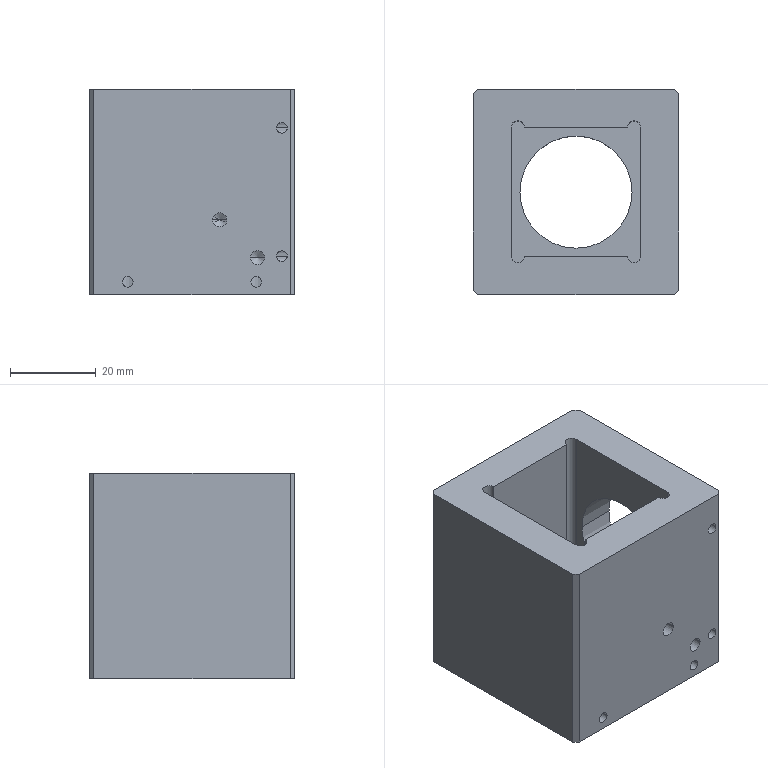NC program | NX | posted with a generic post | part box 48 x 48 x 48 mm
Lines 4993 to 5902 of 9644:
(ZLEVEL_PROFILE_1_COPY , TOOL : D4)
N9954 T11 M6
N9956 G54
N9958 G17 G0 G90 X-12.3 Y-11.259 B0. C0. S8000 M3
N9960 G43 Z30. H11
N9962 Z-0.3
N9964 G94 G1 X-12.9 Y-11.605 F800.
N9966 G3 X-13.1 Y-11.952 R0.4
N9968 G1 Y-13.368
N9970 G2 X-12.1 Y-13.1 R2.
N9972 G1 X-11.887
N9974 G3 X-11.54 Y-12.9 R0.4
N9976 G1 X-11.194 Y-12.3
N9978 G0 X-12.3 Y-11.259 Z-0.6
N9980 G1 X-12.9 Y-11.605
N9982 G3 X-13.1 Y-11.952 R0.4
N9984 G1 Y-13.368
N9986 G2 X-12.1 Y-13.1 R2.
N9988 G1 X-11.887
N9990 G3 X-11.54 Y-12.9 R0.4
N9992 G1 X-11.194 Y-12.3
N9994 G0 X-12.3 Y-11.259 Z-0.9
N9996 G1 X-12.9 Y-11.605
N9998 G3 X-13.1 Y-11.952 R0.4
N10000 G1 Y-13.368
N10002 G2 X-12.1 Y-13.1 R2.
N10004 G1 X-11.887
N10006 G3 X-11.54 Y-12.9 R0.4
N10008 G1 X-11.194 Y-12.3
N10010 G0 X-12.3 Y-11.259 Z-1.2
N10012 G1 X-12.9 Y-11.605
N10014 G3 X-13.1 Y-11.952 R0.4
N10016 G1 Y-13.368
N10018 G2 X-12.1 Y-13.1 R2.
N10020 G1 X-11.887
N10022 G3 X-11.54 Y-12.9 R0.4
N10024 G1 X-11.194 Y-12.3
N10026 G0 X-12.3 Y-11.259 Z-1.5
N10028 G1 X-12.9 Y-11.605
N10030 G3 X-13.1 Y-11.952 R0.4
N10032 G1 Y-13.368
N10034 G2 X-12.1 Y-13.1 R2.
N10036 G1 X-11.887
N10038 G3 X-11.54 Y-12.9 R0.4
N10040 G1 X-11.194 Y-12.3
N10042 G0 X-12.3 Y-11.259 Z-1.8
N10044 G1 X-12.9 Y-11.605
N10046 G3 X-13.1 Y-11.952 R0.4
N10048 G1 Y-13.368
N10050 G2 X-12.1 Y-13.1 R2.
N10052 G1 X-11.887
N10054 G3 X-11.54 Y-12.9 R0.4
N10056 G1 X-11.194 Y-12.3
N10058 G0 X-12.3 Y-11.259 Z-2.1
N10060 G1 X-12.9 Y-11.605
N10062 G3 X-13.1 Y-11.952 R0.4
N10064 G1 Y-13.368
N10066 G2 X-12.1 Y-13.1 R2.
N10068 G1 X-11.887
N10070 G3 X-11.54 Y-12.9 R0.4
N10072 G1 X-11.194 Y-12.3
N10074 G0 X-12.3 Y-11.259 Z-2.4
N10076 G1 X-12.9 Y-11.605
N10078 G3 X-13.1 Y-11.952 R0.4
N10080 G1 Y-13.368
N10082 G2 X-12.1 Y-13.1 R2.
N10084 G1 X-11.887
N10086 G3 X-11.54 Y-12.9 R0.4
N10088 G1 X-11.194 Y-12.3
N10090 G0 X-12.3 Y-11.259 Z-2.7
N10092 G1 X-12.9 Y-11.605
N10094 G3 X-13.1 Y-11.952 R0.4
N10096 G1 Y-13.368
N10098 G2 X-12.1 Y-13.1 R2.
N10100 G1 X-11.887
N10102 G3 X-11.54 Y-12.9 R0.4
N10104 G1 X-11.194 Y-12.3
N10106 G0 X-12.3 Y-11.259 Z-3.
N10108 G1 X-12.9 Y-11.605
N10110 G3 X-13.1 Y-11.952 R0.4
N10112 G1 Y-13.368
N10114 G2 X-12.1 Y-13.1 R2.
N10116 G1 X-11.887
N10118 G3 X-11.54 Y-12.9 R0.4
N10120 G1 X-11.194 Y-12.3
N10122 G0 X-12.3 Y-11.259 Z-3.3
N10124 G1 X-12.9 Y-11.605
N10126 G3 X-13.1 Y-11.952 R0.4
N10128 G1 Y-13.368
N10130 G2 X-12.1 Y-13.1 R2.
N10132 G1 X-11.887
N10134 G3 X-11.54 Y-12.9 R0.4
N10136 G1 X-11.194 Y-12.3
N10138 G0 X-12.3 Y-11.259 Z-3.6
N10140 G1 X-12.9 Y-11.605
N10142 G3 X-13.1 Y-11.952 R0.4
N10144 G1 Y-13.368
N10146 G2 X-12.1 Y-13.1 R2.
N10148 G1 X-11.887
N10150 G3 X-11.54 Y-12.9 R0.4
N10152 G1 X-11.194 Y-12.3
N10154 G0 X-12.3 Y-11.259 Z-3.9
N10156 G1 X-12.9 Y-11.605
N10158 G3 X-13.1 Y-11.952 R0.4
N10160 G1 Y-13.368
N10162 G2 X-12.1 Y-13.1 R2.
N10164 G1 X-11.887
N10166 G3 X-11.54 Y-12.9 R0.4
N10168 G1 X-11.194 Y-12.3
N10170 G0 X-12.3 Y-11.259 Z-4.2
N10172 G1 X-12.9 Y-11.605
N10174 G3 X-13.1 Y-11.952 R0.4
N10176 G1 Y-13.368
N10178 G2 X-12.1 Y-13.1 R2.
N10180 G1 X-11.887
N10182 G3 X-11.54 Y-12.9 R0.4
N10184 G1 X-11.194 Y-12.3
N10186 G0 X-12.3 Y-11.259 Z-4.5
N10188 G1 X-12.9 Y-11.605
N10190 G3 X-13.1 Y-11.952 R0.4
N10192 G1 Y-13.368
N10194 G2 X-12.1 Y-13.1 R2.
N10196 G1 X-11.887
N10198 G3 X-11.54 Y-12.9 R0.4
N10200 G1 X-11.194 Y-12.3
N10202 G0 X-12.3 Y-11.259 Z-4.8
N10204 G1 X-12.9 Y-11.605
N10206 G3 X-13.1 Y-11.952 R0.4
N10208 G1 Y-13.368
N10210 G2 X-12.1 Y-13.1 R2.
N10212 G1 X-11.887
N10214 G3 X-11.54 Y-12.9 R0.4
N10216 G1 X-11.194 Y-12.3
N10218 G0 X-12.3 Y-11.259 Z-5.1
N10220 G1 X-12.9 Y-11.605
N10222 G3 X-13.1 Y-11.952 R0.4
N10224 G1 Y-13.368
N10226 G2 X-12.1 Y-13.1 R2.
N10228 G1 X-11.887
N10230 G3 X-11.54 Y-12.9 R0.4
N10232 G1 X-11.194 Y-12.3
N10234 G0 X-12.3 Y-11.259 Z-5.4
N10236 G1 X-12.9 Y-11.605
N10238 G3 X-13.1 Y-11.951 R0.4
N10240 G1 Y-13.368
N10242 G2 X-12.1 Y-13.1 R2.
N10244 G1 X-11.887
N10246 G3 X-11.54 Y-12.9 R0.4
N10248 G1 X-11.194 Y-12.3
N10250 G0 X-12.3 Y-11.259 Z-5.7
N10252 G1 X-12.9 Y-11.605
N10254 G3 X-13.1 Y-11.951 R0.4
N10256 G1 Y-13.368
N10258 G2 X-12.1 Y-13.1 R2.
N10260 G1 X-11.887
N10262 G3 X-11.54 Y-12.9 R0.4
N10264 G1 X-11.194 Y-12.3
N10266 G0 X-12.3 Y-11.259 Z-6.
N10268 G1 X-12.9 Y-11.605
N10270 G3 X-13.1 Y-11.951 R0.4
N10272 G1 Y-13.368
N10274 G2 X-12.1 Y-13.1 R2.
N10276 G1 X-11.887
N10278 G3 X-11.54 Y-12.9 R0.4
N10280 G1 X-11.194 Y-12.3
N10282 G0 X-12.3 Y-11.259 Z-6.3
N10284 G1 X-12.9 Y-11.605
N10286 G3 X-13.1 Y-11.951 R0.4
N10288 G1 Y-13.368
N10290 G2 X-12.1 Y-13.1 R2.
N10292 G1 X-11.887
N10294 G3 X-11.54 Y-12.9 R0.4
N10296 G1 X-11.194 Y-12.3
N10298 G0 X-12.3 Y-11.259 Z-6.6
N10300 G1 X-12.9 Y-11.605
N10302 G3 X-13.1 Y-11.951 R0.4
N10304 G1 Y-13.368
N10306 G2 X-12.1 Y-13.1 R2.
N10308 G1 X-11.887
N10310 G3 X-11.54 Y-12.9 R0.4
N10312 G1 X-11.194 Y-12.3
N10314 G0 X-12.3 Y-11.259 Z-6.9
N10316 G1 X-12.9 Y-11.605
N10318 G3 X-13.1 Y-11.951 R0.4
N10320 G1 Y-13.368
N10322 G2 X-12.1 Y-13.1 R2.
N10324 G1 X-11.887
N10326 G3 X-11.54 Y-12.9 R0.4
N10328 G1 X-11.194 Y-12.3
N10330 G0 X-12.3 Y-11.259 Z-7.2
N10332 G1 X-12.9 Y-11.605
N10334 G3 X-13.1 Y-11.951 R0.4
N10336 G1 Y-13.368
N10338 G2 X-12.1 Y-13.1 R2.
N10340 G1 X-11.887
N10342 G3 X-11.54 Y-12.9 R0.4
N10344 G1 X-11.194 Y-12.3
N10346 G0 X-12.3 Y-11.259 Z-7.5
N10348 G1 X-12.9 Y-11.605
N10350 G3 X-13.1 Y-11.951 R0.4
N10352 G1 Y-13.368
N10354 G2 X-12.1 Y-13.1 R2.
N10356 G1 X-11.887
N10358 G3 X-11.54 Y-12.9 R0.4
N10360 G1 X-11.194 Y-12.3
N10362 G0 X-12.3 Y-11.259 Z-7.8
N10364 G1 X-12.9 Y-11.605
N10366 G3 X-13.1 Y-11.951 R0.4
N10368 G1 Y-13.368
N10370 G2 X-12.1 Y-13.1 R2.
N10372 G1 X-11.887
N10374 G3 X-11.54 Y-12.9 R0.4
N10376 G1 X-11.194 Y-12.3
N10378 G0 X-12.3 Y-11.259 Z-8.1
N10380 G1 X-12.9 Y-11.605
N10382 G3 X-13.1 Y-11.951 R0.4
N10384 G1 Y-13.368
N10386 G2 X-12.1 Y-13.1 R2.
N10388 G1 X-11.887
N10390 G3 X-11.54 Y-12.9 R0.4
N10392 G1 X-11.194 Y-12.3
N10394 G0 X-12.3 Y-11.259 Z-8.4
N10396 G1 X-12.9 Y-11.605
N10398 G3 X-13.1 Y-11.951 R0.4
N10400 G1 Y-13.368
N10402 G2 X-12.1 Y-13.1 R2.
N10404 G1 X-11.887
N10406 G3 X-11.54 Y-12.9 R0.4
N10408 G1 X-11.194 Y-12.3
N10410 G0 X-12.3 Y-11.259 Z-8.7
N10412 G1 X-12.9 Y-11.605
N10414 G3 X-13.1 Y-11.951 R0.4
N10416 G1 Y-13.368
N10418 G2 X-12.1 Y-13.1 R2.
N10420 G1 X-11.887
N10422 G3 X-11.54 Y-12.9 R0.4
N10424 G1 X-11.194 Y-12.3
N10426 G0 X-12.3 Y-11.259 Z-9.
N10428 G1 X-12.9 Y-11.605
N10430 G3 X-13.1 Y-11.951 R0.4
N10432 G1 Y-13.368
N10434 G2 X-12.1 Y-13.1 R2.
N10436 G1 X-11.887
N10438 G3 X-11.54 Y-12.9 R0.4
N10440 G1 X-11.194 Y-12.3
N10442 G0 X-12.3 Y-11.259 Z-9.3
N10444 G1 X-12.9 Y-11.605
N10446 G3 X-13.1 Y-11.951 R0.4
N10448 G1 Y-13.368
N10450 G2 X-12.1 Y-13.1 R2.
N10452 G1 X-11.887
N10454 G3 X-11.54 Y-12.9 R0.4
N10456 G1 X-11.194 Y-12.3
N10458 G0 X-12.3 Y-11.259 Z-9.6
N10460 G1 X-12.9 Y-11.605
N10462 G3 X-13.1 Y-11.951 R0.4
N10464 G1 Y-13.368
N10466 G2 X-12.1 Y-13.1 R2.
N10468 G1 X-11.887
N10470 G3 X-11.54 Y-12.9 R0.4
N10472 G1 X-11.194 Y-12.3
N10474 G0 X-12.3 Y-11.259 Z-9.9
N10476 G1 X-12.9 Y-11.605
N10478 G3 X-13.1 Y-11.951 R0.4
N10480 G1 Y-13.368
N10482 G2 X-12.1 Y-13.1 R2.
N10484 G1 X-11.887
N10486 G3 X-11.54 Y-12.9 R0.4
N10488 G1 X-11.194 Y-12.3
N10490 G0 X-12.3 Y-11.259 Z-10.2
N10492 G1 X-12.9 Y-11.605
N10494 G3 X-13.1 Y-11.951 R0.4
N10496 G1 Y-13.368
N10498 G2 X-12.1 Y-13.1 R2.
N10500 G1 X-11.887
N10502 G3 X-11.54 Y-12.9 R0.4
N10504 G1 X-11.194 Y-12.3
N10506 G0 X-12.3 Y-11.259 Z-10.5
N10508 G1 X-12.9 Y-11.605
N10510 G3 X-13.1 Y-11.951 R0.4
N10512 G1 Y-13.368
N10514 G2 X-12.1 Y-13.1 R2.
N10516 G1 X-11.887
N10518 G3 X-11.54 Y-12.9 R0.4
N10520 G1 X-11.194 Y-12.3
N10522 G0 X-12.3 Y-11.259 Z-10.8
N10524 G1 X-12.9 Y-11.605
N10526 G3 X-13.1 Y-11.951 R0.4
N10528 G1 Y-13.368
N10530 G2 X-12.1 Y-13.1 R2.
N10532 G1 X-11.887
N10534 G3 X-11.54 Y-12.9 R0.4
N10536 G1 X-11.194 Y-12.3
N10538 G0 X-12.3 Y-11.259 Z-11.1
N10540 G1 X-12.9 Y-11.605
N10542 G3 X-13.1 Y-11.951 R0.4
N10544 G1 Y-13.368
N10546 G2 X-12.1 Y-13.1 R2.
N10548 G1 X-11.887
N10550 G3 X-11.54 Y-12.9 R0.4
N10552 G1 X-11.194 Y-12.3
N10554 G0 X-12.3 Y-11.259 Z-11.4
N10556 G1 X-12.9 Y-11.605
N10558 G3 X-13.1 Y-11.951 R0.4
N10560 G1 Y-13.368
N10562 G2 X-12.1 Y-13.1 R2.
N10564 G1 X-11.887
N10566 G3 X-11.54 Y-12.9 R0.4
N10568 G1 X-11.194 Y-12.3
N10570 G0 X-12.3 Y-11.259 Z-11.7
N10572 G1 X-12.9 Y-11.605
N10574 G3 X-13.1 Y-11.951 R0.4
N10576 G1 Y-13.368
N10578 G2 X-12.1 Y-13.1 R2.
N10580 G1 X-11.887
N10582 G3 X-11.54 Y-12.9 R0.4
N10584 G1 X-11.194 Y-12.3
N10586 G0 X-12.3 Y-11.259 Z-12.
N10588 G1 X-12.9 Y-11.605
N10590 G3 X-13.1 Y-11.951 R0.4
N10592 G1 Y-13.368
N10594 G2 X-12.1 Y-13.1 R2.
N10596 G1 X-11.887
N10598 G3 X-11.54 Y-12.9 R0.4
N10600 G1 X-11.194 Y-12.3
N10602 G0 X-12.3 Y-11.259 Z-12.3
N10604 G1 X-12.9 Y-11.605
N10606 G3 X-13.1 Y-11.951 R0.4
N10608 G1 Y-13.368
N10610 G2 X-12.1 Y-13.1 R2.
N10612 G1 X-11.887
N10614 G3 X-11.54 Y-12.9 R0.4
N10616 G1 X-11.194 Y-12.3
N10618 G0 X-12.3 Y-11.259 Z-12.6
N10620 G1 X-12.9 Y-11.605
N10622 G3 X-13.1 Y-11.951 R0.4
N10624 G1 Y-13.368
N10626 G2 X-12.1 Y-13.1 R2.
N10628 G1 X-11.887
N10630 G3 X-11.54 Y-12.9 R0.4
N10632 G1 X-11.194 Y-12.3
N10634 G0 X-12.3 Y-11.259 Z-12.9
N10636 G1 X-12.9 Y-11.605
N10638 G3 X-13.1 Y-11.951 R0.4
N10640 G1 Y-13.368
N10642 G2 X-12.1 Y-13.1 R2.
N10644 G1 X-11.887
N10646 G3 X-11.54 Y-12.9 R0.4
N10648 G1 X-11.194 Y-12.3
N10650 G0 X-12.3 Y-11.259 Z-13.2
N10652 G1 X-12.9 Y-11.605
N10654 G3 X-13.1 Y-11.951 R0.4
N10656 G1 Y-13.368
N10658 G2 X-12.1 Y-13.1 R2.
N10660 G1 X-11.887
N10662 G3 X-11.54 Y-12.9 R0.4
N10664 G1 X-11.194 Y-12.3
N10666 G0 X-12.3 Y-11.259 Z-13.5
N10668 G1 X-12.9 Y-11.605
N10670 G3 X-13.1 Y-11.951 R0.4
N10672 G1 Y-13.368
N10674 G2 X-12.1 Y-13.1 R2.
N10676 G1 X-11.887
N10678 G3 X-11.54 Y-12.9 R0.4
N10680 G1 X-11.194 Y-12.3
N10682 G0 X-12.3 Y-11.259 Z-13.8
N10684 G1 X-12.9 Y-11.605
N10686 G3 X-13.1 Y-11.951 R0.4
N10688 G1 Y-13.368
N10690 G2 X-12.1 Y-13.1 R2.
N10692 G1 X-11.887
N10694 G3 X-11.54 Y-12.9 R0.4
N10696 G1 X-11.194 Y-12.3
N10698 G0 X-12.3 Y-11.259 Z-14.1
N10700 G1 X-12.9 Y-11.605
N10702 G3 X-13.1 Y-11.951 R0.4
N10704 G1 Y-13.368
N10706 G2 X-12.1 Y-13.1 R2.
N10708 G1 X-11.887
N10710 G3 X-11.54 Y-12.9 R0.4
N10712 G1 X-11.194 Y-12.3
N10714 G0 X-12.3 Y-11.259 Z-14.4
N10716 G1 X-12.9 Y-11.605
N10718 G3 X-13.1 Y-11.951 R0.4
N10720 G1 Y-13.368
N10722 G2 X-12.1 Y-13.1 R2.
N10724 G1 X-11.887
N10726 G3 X-11.54 Y-12.9 R0.4
N10728 G1 X-11.194 Y-12.3
N10730 G0 X-12.3 Y-11.259 Z-14.7
N10732 G1 X-12.9 Y-11.605
N10734 G3 X-13.1 Y-11.951 R0.4
N10736 G1 Y-13.368
N10738 G2 X-12.1 Y-13.1 R2.
N10740 G1 X-11.887
N10742 G3 X-11.54 Y-12.9 R0.4
N10744 G1 X-11.194 Y-12.3
N10746 G0 X-12.3 Y-11.259 Z-15.
N10748 G1 X-12.9 Y-11.605
N10750 G3 X-13.1 Y-11.951 R0.4
N10752 G1 Y-13.368
N10754 G2 X-12.1 Y-13.1 R2.
N10756 G1 X-11.887
N10758 G3 X-11.54 Y-12.9 R0.4
N10760 G1 X-11.194 Y-12.3
N10762 G0 X-12.3 Y-11.259 Z-15.3
N10764 G1 X-12.9 Y-11.605
N10766 G3 X-13.1 Y-11.951 R0.4
N10768 G1 Y-13.368
N10770 G2 X-12.1 Y-13.1 R2.
N10772 G1 X-11.887
N10774 G3 X-11.54 Y-12.9 R0.4
N10776 G1 X-11.194 Y-12.3
N10778 G0 X-12.3 Y-11.259 Z-15.6
N10780 G1 X-12.9 Y-11.605
N10782 G3 X-13.1 Y-11.951 R0.4
N10784 G1 Y-13.368
N10786 G2 X-12.1 Y-13.1 R2.
N10788 G1 X-11.887
N10790 G3 X-11.54 Y-12.9 R0.4
N10792 G1 X-11.194 Y-12.3
N10794 G0 X-12.3 Y-11.259 Z-15.9
N10796 G1 X-12.9 Y-11.605
N10798 G3 X-13.1 Y-11.951 R0.4
N10800 G1 Y-13.368
N10802 G2 X-12.1 Y-13.1 R2.
N10804 G1 X-11.887
N10806 G3 X-11.54 Y-12.9 R0.4
N10808 G1 X-11.194 Y-12.3
N10810 G0 X-12.3 Y-11.259 Z-16.2
N10812 G1 X-12.9 Y-11.605
N10814 G3 X-13.1 Y-11.951 R0.4
N10816 G1 Y-13.368
N10818 G2 X-12.1 Y-13.1 R2.
N10820 G1 X-11.887
N10822 G3 X-11.54 Y-12.9 R0.4
N10824 G1 X-11.194 Y-12.3
N10826 G0 X-12.3 Y-11.259 Z-16.5
N10828 G1 X-12.9 Y-11.605
N10830 G3 X-13.1 Y-11.951 R0.4
N10832 G1 Y-13.368
N10834 G2 X-12.1 Y-13.1 R2.
N10836 G1 X-11.887
N10838 G3 X-11.54 Y-12.9 R0.4
N10840 G1 X-11.194 Y-12.3
N10842 G0 X-12.3 Y-11.259 Z-16.8
N10844 G1 X-12.9 Y-11.605
N10846 G3 X-13.1 Y-11.951 R0.4
N10848 G1 Y-13.368
N10850 G2 X-12.1 Y-13.1 R2.
N10852 G1 X-11.887
N10854 G3 X-11.54 Y-12.9 R0.4
N10856 G1 X-11.194 Y-12.3
N10858 G0 X-12.3 Y-11.259 Z-17.1
N10860 G1 X-12.9 Y-11.605
N10862 G3 X-13.1 Y-11.951 R0.4
N10864 G1 Y-13.368
N10866 G2 X-12.1 Y-13.1 R2.
N10868 G1 X-11.887
N10870 G3 X-11.54 Y-12.9 R0.4
N10872 G1 X-11.194 Y-12.3
N10874 G0 X-12.3 Y-11.259 Z-17.4
N10876 G1 X-12.9 Y-11.605
N10878 G3 X-13.1 Y-11.951 R0.4
N10880 G1 Y-13.368
N10882 G2 X-12.1 Y-13.1 R2.
N10884 G1 X-11.887
N10886 G3 X-11.54 Y-12.9 R0.4
N10888 G1 X-11.194 Y-12.3
N10890 G0 X-12.3 Y-11.259 Z-17.7
N10892 G1 X-12.9 Y-11.605
N10894 G3 X-13.1 Y-11.951 R0.4
N10896 G1 Y-13.368
N10898 G2 X-12.1 Y-13.1 R2.
N10900 G1 X-11.887
N10902 G3 X-11.54 Y-12.9 R0.4
N10904 G1 X-11.194 Y-12.3
N10906 G0 X-12.3 Y-11.259 Z-18.
N10908 G1 X-12.9 Y-11.605
N10910 G3 X-13.1 Y-11.951 R0.4
N10912 G1 Y-13.368
N10914 G2 X-12.1 Y-13.1 R2.
N10916 G1 X-11.887
N10918 G3 X-11.54 Y-12.9 R0.4
N10920 G1 X-11.194 Y-12.3
N10922 G0 X-12.3 Y-11.259 Z-18.3
N10924 G1 X-12.9 Y-11.605
N10926 G3 X-13.1 Y-11.951 R0.4
N10928 G1 Y-13.368
N10930 G2 X-12.1 Y-13.1 R2.
N10932 G1 X-11.887
N10934 G3 X-11.54 Y-12.9 R0.4
N10936 G1 X-11.194 Y-12.3
N10938 G0 X-12.3 Y-11.259 Z-18.6
N10940 G1 X-12.9 Y-11.605
N10942 G3 X-13.1 Y-11.951 R0.4
N10944 G1 Y-13.368
N10946 G2 X-12.1 Y-13.1 R2.
N10948 G1 X-11.887
N10950 G3 X-11.54 Y-12.9 R0.4
N10952 G1 X-11.194 Y-12.3
N10954 G0 X-12.3 Y-11.259 Z-18.9
N10956 G1 X-12.9 Y-11.605
N10958 G3 X-13.1 Y-11.951 R0.4
N10960 G1 Y-13.368
N10962 G2 X-12.1 Y-13.1 R2.
N10964 G1 X-11.887
N10966 G3 X-11.54 Y-12.9 R0.4
N10968 G1 X-11.194 Y-12.3
N10970 G0 X-12.3 Y-11.258 Z-19.2
N10972 G1 X-12.9 Y-11.605
N10974 G3 X-13.1 Y-11.951 R0.4
N10976 G1 Y-13.368
N10978 G2 X-12.1 Y-13.1 R2.
N10980 G1 X-11.887
N10982 G3 X-11.54 Y-12.9 R0.4
N10984 G1 X-11.194 Y-12.3
N10986 G0 X-12.3 Y-11.258 Z-19.5
N10988 G1 X-12.9 Y-11.605
N10990 G3 X-13.1 Y-11.951 R0.4
N10992 G1 Y-13.368
N10994 G2 X-12.1 Y-13.1 R2.
N10996 G1 X-11.887
N10998 G3 X-11.54 Y-12.9 R0.4
N11000 G1 X-11.194 Y-12.3
N11002 G0 X-12.3 Y-11.258 Z-19.8
N11004 G1 X-12.9 Y-11.605
N11006 G3 X-13.1 Y-11.951 R0.4
N11008 G1 Y-13.368
N11010 G2 X-12.1 Y-13.1 R2.
N11012 G1 X-11.887
N11014 G3 X-11.54 Y-12.9 R0.4
N11016 G1 X-11.194 Y-12.3
N11018 G0 X-12.3 Y-11.258 Z-20.1
N11020 G1 X-12.9 Y-11.605
N11022 G3 X-13.1 Y-11.951 R0.4
N11024 G1 Y-13.368
N11026 G2 X-12.1 Y-13.1 R2.
N11028 G1 X-11.887
N11030 G3 X-11.54 Y-12.9 R0.4
N11032 G1 X-11.194 Y-12.3
N11034 G0 X-12.3 Y-11.258 Z-20.4
N11036 G1 X-12.9 Y-11.605
N11038 G3 X-13.1 Y-11.951 R0.4
N11040 G1 Y-13.368
N11042 G2 X-12.1 Y-13.1 R2.
N11044 G1 X-11.887
N11046 G3 X-11.54 Y-12.9 R0.4
N11048 G1 X-11.194 Y-12.3
N11050 G0 X-12.3 Y-11.258 Z-20.7
N11052 G1 X-12.9 Y-11.605
N11054 G3 X-13.1 Y-11.951 R0.4
N11056 G1 Y-13.368
N11058 G2 X-12.1 Y-13.1 R2.
N11060 G1 X-11.887
N11062 G3 X-11.54 Y-12.9 R0.4
N11064 G1 X-11.194 Y-12.3
N11066 G0 X-12.3 Y-11.258 Z-21.
N11068 G1 X-12.9 Y-11.605
N11070 G3 X-13.1 Y-11.951 R0.4
N11072 G1 Y-13.368
N11074 G2 X-12.1 Y-13.1 R2.
N11076 G1 X-11.887
N11078 G3 X-11.54 Y-12.9 R0.4
N11080 G1 X-11.194 Y-12.3
N11082 G0 X-12.3 Y-11.258 Z-21.3
N11084 G1 X-12.9 Y-11.605
N11086 G3 X-13.1 Y-11.951 R0.4
N11088 G1 Y-13.368
N11090 G2 X-12.1 Y-13.1 R2.
N11092 G1 X-11.887
N11094 G3 X-11.54 Y-12.9 R0.4
N11096 G1 X-11.194 Y-12.3
N11098 G0 X-12.3 Y-11.258 Z-21.6
N11100 G1 X-12.9 Y-11.605
N11102 G3 X-13.1 Y-11.951 R0.4
N11104 G1 Y-13.368
N11106 G2 X-12.1 Y-13.1 R2.
N11108 G1 X-11.887
N11110 G3 X-11.54 Y-12.9 R0.4
N11112 G1 X-11.194 Y-12.3
N11114 G0 X-12.3 Y-11.258 Z-21.9
N11116 G1 X-12.9 Y-11.605
N11118 G3 X-13.1 Y-11.951 R0.4
N11120 G1 Y-13.368
N11122 G2 X-12.1 Y-13.1 R2.
N11124 G1 X-11.887
N11126 G3 X-11.54 Y-12.9 R0.4
N11128 G1 X-11.194 Y-12.3
N11130 G0 X-12.3 Y-11.258 Z-22.2
N11132 G1 X-12.9 Y-11.605
N11134 G3 X-13.1 Y-11.951 R0.4
N11136 G1 Y-13.368
N11138 G2 X-12.1 Y-13.1 R2.
N11140 G1 X-11.887
N11142 G3 X-11.54 Y-12.9 R0.4
N11144 G1 X-11.194 Y-12.3
N11146 G0 X-12.3 Y-11.258 Z-22.5
N11148 G1 X-12.9 Y-11.605
N11150 G3 X-13.1 Y-11.951 R0.4
N11152 G1 Y-13.368
N11154 G2 X-12.1 Y-13.1 R2.
N11156 G1 X-11.887
N11158 G3 X-11.54 Y-12.9 R0.4
N11160 G1 X-11.194 Y-12.3
N11162 G0 X-12.3 Y-11.258 Z-22.8
N11164 G1 X-12.9 Y-11.605
N11166 G3 X-13.1 Y-11.951 R0.4
N11168 G1 Y-13.368
N11170 G2 X-12.1 Y-13.1 R2.
N11172 G1 X-11.887
N11174 G3 X-11.54 Y-12.9 R0.4
N11176 G1 X-11.194 Y-12.3
N11178 G0 X-12.3 Y-11.258 Z-23.1
N11180 G1 X-12.9 Y-11.605
N11182 G3 X-13.1 Y-11.951 R0.4
N11184 G1 Y-13.368
N11186 G2 X-12.1 Y-13.1 R2.
N11188 G1 X-11.887
N11190 G3 X-11.54 Y-12.9 R0.4
N11192 G1 X-11.194 Y-12.3
N11194 G0 X-12.3 Y-11.258 Z-23.4
N11196 G1 X-12.9 Y-11.605
N11198 G3 X-13.1 Y-11.951 R0.4
N11200 G1 Y-13.368
N11202 G2 X-12.1 Y-13.1 R2.
N11204 G1 X-11.887
N11206 G3 X-11.54 Y-12.9 R0.4
N11208 G1 X-11.194 Y-12.3
N11210 G0 X-12.3 Y-11.258 Z-23.7
N11212 G1 X-12.9 Y-11.605
N11214 G3 X-13.1 Y-11.951 R0.4
N11216 G1 Y-13.368
N11218 G2 X-12.1 Y-13.1 R2.
N11220 G1 X-11.887
N11222 G3 X-11.54 Y-12.9 R0.4
N11224 G1 X-11.194 Y-12.3
N11226 G0 X-12.3 Y-11.258 Z-24.
N11228 G1 X-12.9 Y-11.605
N11230 G3 X-13.1 Y-11.951 R0.4
N11232 G1 Y-13.368
N11234 G2 X-12.1 Y-13.1 R2.
N11236 G1 X-11.887
N11238 G3 X-11.54 Y-12.9 R0.4
N11240 G1 X-11.194 Y-12.3
N11242 G0 X-12.3 Y-11.258 Z-24.3
N11244 G1 X-12.9 Y-11.605
N11246 G3 X-13.1 Y-11.951 R0.4
N11248 G1 Y-13.368
N11250 G2 X-12.1 Y-13.1 R2.
N11252 G1 X-11.887
N11254 G3 X-11.54 Y-12.9 R0.4
N11256 G1 X-11.194 Y-12.3
N11258 G0 X-12.3 Y-11.258 Z-24.6
N11260 G1 X-12.9 Y-11.605
N11262 G3 X-13.1 Y-11.951 R0.4
N11264 G1 Y-13.368
N11266 G2 X-12.1 Y-13.1 R2.
N11268 G1 X-11.887
N11270 G3 X-11.54 Y-12.9 R0.4
N11272 G1 X-11.194 Y-12.3
N11274 G0 X-12.3 Y-11.258 Z-24.9
N11276 G1 X-12.9 Y-11.605
N11278 G3 X-13.1 Y-11.951 R0.4
N11280 G1 Y-13.368
N11282 G2 X-12.1 Y-13.1 R2.
N11284 G1 X-11.887
N11286 G3 X-11.54 Y-12.9 R0.4
N11288 G1 X-11.194 Y-12.3
N11290 G0 X-12.3 Y-11.258 Z-25.2
N11292 G1 X-12.9 Y-11.605
N11294 G3 X-13.1 Y-11.951 R0.4
N11296 G1 Y-13.368
N11298 G2 X-12.1 Y-13.1 R2.
N11300 G1 X-11.887
N11302 G3 X-11.54 Y-12.9 R0.4
N11304 G1 X-11.194 Y-12.3
N11306 G0 X-12.3 Y-11.258 Z-25.5
N11308 G1 X-12.9 Y-11.605
N11310 G3 X-13.1 Y-11.951 R0.4
N11312 G1 Y-13.368
N11314 G2 X-12.1 Y-13.1 R2.
N11316 G1 X-11.887
N11318 G3 X-11.54 Y-12.9 R0.4
N11320 G1 X-11.194 Y-12.3
N11322 G0 X-12.3 Y-11.258 Z-25.8
N11324 G1 X-12.9 Y-11.605
N11326 G3 X-13.1 Y-11.951 R0.4
N11328 G1 Y-13.368
N11330 G2 X-12.1 Y-13.1 R2.
N11332 G1 X-11.887
N11334 G3 X-11.54 Y-12.9 R0.4
N11336 G1 X-11.194 Y-12.3
N11338 G0 X-12.3 Y-11.258 Z-26.1
N11340 G1 X-12.9 Y-11.605
N11342 G3 X-13.1 Y-11.951 R0.4
N11344 G1 Y-13.368
N11346 G2 X-12.1 Y-13.1 R2.
N11348 G1 X-11.887
N11350 G3 X-11.54 Y-12.9 R0.4
N11352 G1 X-11.194 Y-12.3
N11354 G0 X-12.3 Y-11.258 Z-26.4
N11356 G1 X-12.9 Y-11.605
N11358 G3 X-13.1 Y-11.951 R0.4
N11360 G1 Y-13.368
N11362 G2 X-12.1 Y-13.1 R2.
N11364 G1 X-11.887
N11366 G3 X-11.54 Y-12.9 R0.4
N11368 G1 X-11.194 Y-12.3
N11370 G0 X-12.3 Y-11.258 Z-26.7
N11372 G1 X-12.9 Y-11.605
N11374 G3 X-13.1 Y-11.951 R0.4
N11376 G1 Y-13.368
N11378 G2 X-12.1 Y-13.1 R2.
N11380 G1 X-11.887
N11382 G3 X-11.54 Y-12.9 R0.4
N11384 G1 X-11.194 Y-12.3
N11386 G0 X-12.3 Y-11.258 Z-27.
N11388 G1 X-12.9 Y-11.605
N11390 G3 X-13.1 Y-11.951 R0.4
N11392 G1 Y-13.368
N11394 G2 X-12.1 Y-13.1 R2.
N11396 G1 X-11.887
N11398 G3 X-11.54 Y-12.9 R0.4
N11400 G1 X-11.194 Y-12.3
N11402 G0 X-12.3 Y-11.258 Z-27.3
N11404 G1 X-12.9 Y-11.605
N11406 G3 X-13.1 Y-11.951 R0.4
N11408 G1 Y-13.368
N11410 G2 X-12.1 Y-13.1 R2.
N11412 G1 X-11.887
N11414 G3 X-11.54 Y-12.9 R0.4
N11416 G1 X-11.194 Y-12.3
N11418 G0 X-12.3 Y-11.258 Z-27.6
N11420 G1 X-12.9 Y-11.605
N11422 G3 X-13.1 Y-11.951 R0.4
N11424 G1 Y-13.368
N11426 G2 X-12.1 Y-13.1 R2.
N11428 G1 X-11.886
N11430 G3 X-11.54 Y-12.9 R0.4
N11432 G1 X-11.194 Y-12.3
N11434 G0 X-12.3 Y-11.258 Z-27.9
N11436 G1 X-12.9 Y-11.605
N11438 G3 X-13.1 Y-11.951 R0.4
N11440 G1 Y-13.368
N11442 G2 X-12.1 Y-13.1 R2.
N11444 G1 X-11.886
N11446 G3 X-11.54 Y-12.9 R0.4
N11448 G1 X-11.194 Y-12.3
N11450 G0 X-12.3 Y-11.258 Z-28.2
N11452 G1 X-12.9 Y-11.605
N11454 G3 X-13.1 Y-11.951 R0.4
N11456 G1 Y-13.368
N11458 G2 X-12.1 Y-13.1 R2.
N11460 G1 X-11.886
N11462 G3 X-11.54 Y-12.9 R0.4
N11464 G1 X-11.194 Y-12.3
N11466 G0 X-12.3 Y-11.258 Z-28.5
N11468 G1 X-12.9 Y-11.605
N11470 G3 X-13.1 Y-11.951 R0.4
N11472 G1 Y-13.368
N11474 G2 X-12.1 Y-13.1 R2.
N11476 G1 X-11.886
N11478 G3 X-11.54 Y-12.9 R0.4
N11480 G1 X-11.194 Y-12.3
N11482 G0 X-12.3 Y-11.258 Z-28.8
N11484 G1 X-12.9 Y-11.605
N11486 G3 X-13.1 Y-11.951 R0.4
N11488 G1 Y-13.368
N11490 G2 X-12.1 Y-13.1 R2.
N11492 G1 X-11.886
N11494 G3 X-11.54 Y-12.9 R0.4
N11496 G1 X-11.194 Y-12.3
N11498 G0 X-12.3 Y-11.258 Z-29.1
N11500 G1 X-12.9 Y-11.605
N11502 G3 X-13.1 Y-11.951 R0.4
N11504 G1 Y-13.368
N11506 G2 X-12.1 Y-13.1 R2.
N11508 G1 X-11.886
N11510 G3 X-11.54 Y-12.9 R0.4
N11512 G1 X-11.194 Y-12.3
N11514 G0 X-12.3 Y-11.258 Z-29.4
N11516 G1 X-12.9 Y-11.605
N11518 G3 X-13.1 Y-11.951 R0.4
N11520 G1 Y-13.368
N11522 G2 X-12.1 Y-13.1 R2.
N11524 G1 X-11.886
N11526 G3 X-11.54 Y-12.9 R0.4
N11528 G1 X-11.194 Y-12.3
N11530 G0 X-12.3 Y-11.258 Z-29.7
N11532 G1 X-12.9 Y-11.605
N11534 G3 X-13.1 Y-11.951 R0.4
N11536 G1 Y-13.368
N11538 G2 X-12.1 Y-13.1 R2.
N11540 G1 X-11.886
N11542 G3 X-11.54 Y-12.9 R0.4
N11544 G1 X-11.194 Y-12.3
N11546 G0 X-12.3 Y-11.258 Z-30.
N11548 G1 X-12.9 Y-11.605
N11550 G3 X-13.1 Y-11.951 R0.4
N11552 G1 Y-13.368
N11554 G2 X-12.1 Y-13.1 R2.
N11556 G1 X-11.886
N11558 G3 X-11.54 Y-12.9 R0.4
N11560 G1 X-11.194 Y-12.3
N11562 G0 X-12.3 Y-11.258 Z-30.3
N11564 G1 X-12.9 Y-11.605
N11566 G3 X-13.1 Y-11.951 R0.4
N11568 G1 Y-13.368
N11570 G2 X-12.1 Y-13.1 R2.
N11572 G1 X-11.886
N11574 G3 X-11.54 Y-12.9 R0.4
N11576 G1 X-11.194 Y-12.3
N11578 G0 X-12.3 Y-11.258 Z-30.6
N11580 G1 X-12.9 Y-11.605
N11582 G3 X-13.1 Y-11.951 R0.4
N11584 G1 Y-13.368
N11586 G2 X-12.1 Y-13.1 R2.
N11588 G1 X-11.886
N11590 G3 X-11.54 Y-12.9 R0.4
N11592 G1 X-11.194 Y-12.3
N11594 G0 X-12.3 Y-11.258 Z-30.9
N11596 G1 X-12.9 Y-11.605
N11598 G3 X-13.1 Y-11.951 R0.4
N11600 G1 Y-13.368
N11602 G2 X-12.1 Y-13.1 R2.
N11604 G1 X-11.886
N11606 G3 X-11.54 Y-12.9 R0.4
N11608 G1 X-11.194 Y-12.3
N11610 G0 X-12.3 Y-11.258 Z-31.2
N11612 G1 X-12.9 Y-11.605
N11614 G3 X-13.1 Y-11.951 R0.4
N11616 G1 Y-13.368
N11618 G2 X-12.1 Y-13.1 R2.
N11620 G1 X-11.886
N11622 G3 X-11.54 Y-12.9 R0.4
N11624 G1 X-11.194 Y-12.3
N11626 G0 X-12.3 Y-11.258 Z-31.5
N11628 G1 X-12.9 Y-11.605
N11630 G3 X-13.1 Y-11.951 R0.4
N11632 G1 Y-13.368
N11634 G2 X-12.1 Y-13.1 R2.
N11636 G1 X-11.886
N11638 G3 X-11.54 Y-12.9 R0.4
N11640 G1 X-11.194 Y-12.3
N11642 G0 X-12.3 Y-11.258 Z-31.8
N11644 G1 X-12.9 Y-11.605
N11646 G3 X-13.1 Y-11.951 R0.4
N11648 G1 Y-13.368
N11650 G2 X-12.1 Y-13.1 R2.
N11652 G1 X-11.886
N11654 G3 X-11.54 Y-12.9 R0.4
N11656 G1 X-11.194 Y-12.3
N11658 G0 X-12.3 Y-11.258 Z-32.1
N11660 G1 X-12.9 Y-11.605
N11662 G3 X-13.1 Y-11.951 R0.4
N11664 G1 Y-13.368
N11666 G2 X-12.1 Y-13.1 R2.
N11668 G1 X-11.886
N11670 G3 X-11.54 Y-12.9 R0.4
N11672 G1 X-11.194 Y-12.3
N11674 G0 X-12.3 Y-11.258 Z-32.4
N11676 G1 X-12.9 Y-11.605
N11678 G3 X-13.1 Y-11.951 R0.4
N11680 G1 Y-13.368
N11682 G2 X-12.1 Y-13.1 R2.
N11684 G1 X-11.886
N11686 G3 X-11.54 Y-12.9 R0.4
N11688 G1 X-11.194 Y-12.3
N11690 G0 X-12.3 Y-11.258 Z-32.7
N11692 G1 X-12.9 Y-11.605
N11694 G3 X-13.1 Y-11.951 R0.4
N11696 G1 Y-13.368
N11698 G2 X-12.1 Y-13.1 R2.
N11700 G1 X-11.886
N11702 G3 X-11.54 Y-12.9 R0.4
N11704 G1 X-11.194 Y-12.3
N11706 G0 X-12.3 Y-11.258 Z-33.
N11708 G1 X-12.9 Y-11.605
N11710 G3 X-13.1 Y-11.951 R0.4
N11712 G1 Y-13.368
N11714 G2 X-12.1 Y-13.1 R2.
N11716 G1 X-11.886
N11718 G3 X-11.54 Y-12.9 R0.4
N11720 G1 X-11.194 Y-12.3
N11722 G0 X-12.3 Y-11.258 Z-33.3
N11724 G1 X-12.9 Y-11.605
N11726 G3 X-13.1 Y-11.951 R0.4
N11728 G1 Y-13.368
N11730 G2 X-12.1 Y-13.1 R2.
N11732 G1 X-11.886
N11734 G3 X-11.54 Y-12.9 R0.4
N11736 G1 X-11.194 Y-12.3
N11738 G0 X-12.3 Y-11.258 Z-33.6
N11740 G1 X-12.9 Y-11.605
N11742 G3 X-13.1 Y-11.951 R0.4
N11744 G1 Y-13.368
N11746 G2 X-12.1 Y-13.1 R2.
N11748 G1 X-11.886
N11750 G3 X-11.54 Y-12.9 R0.4
N11752 G1 X-11.194 Y-12.3
N11754 G0 X-12.3 Y-11.258 Z-33.9
N11756 G1 X-12.9 Y-11.605
N11758 G3 X-13.1 Y-11.951 R0.4
N11760 G1 Y-13.368
N11762 G2 X-12.1 Y-13.1 R2.
N11764 G1 X-11.886
N11766 G3 X-11.54 Y-12.9 R0.4